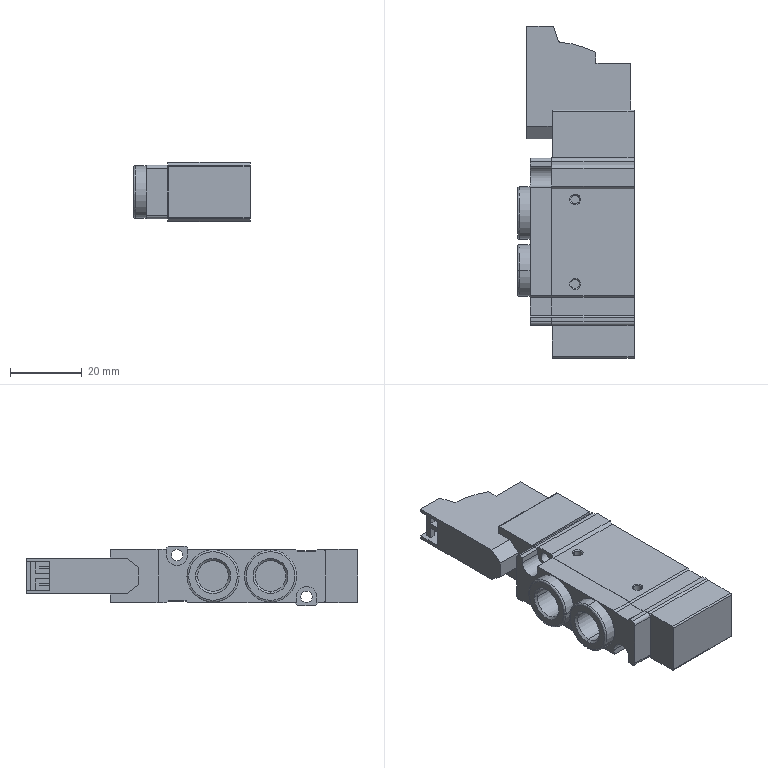Part | STEP file | Solenoid valve 7V110-06-B terminal type cable length 0.5m | 1 solid | 157 faces | box 32.5 x 92.3 x 16.6 mm | volume 31794 mm3 | plane 99 | cylinder 40 | cone 14 | spline 4 | commonest cylinder face diameters 8.566 x10 2 x8 0.8 x4 2.459 x4 3.2 x4 14.5 x4